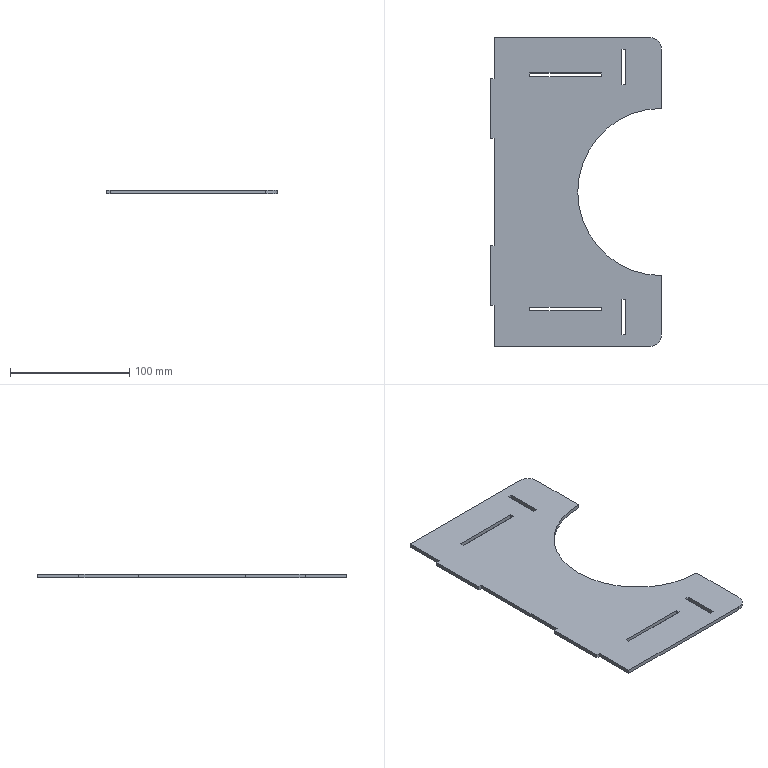Part | SolidWorks | features FlatPattern 1, SMBaseFlange 1, SheetMetal 1 | 1 solid | 34 faces | box 143.5 x 260 x 3.2 mm | volume 91069 mm3 | plane 31 | cylinder 3 | commonest cylinder face diameters 20 x2 140.5 x1
STEP:
#1=CARTESIAN_POINT('',(140.5,109.865,0.));
#2=VERTEX_POINT('',#1);
#3=CARTESIAN_POINT('',(130.5,119.865,0.));
#4=VERTEX_POINT('',#3);
#5=CARTESIAN_POINT('',(130.5,109.865,0.));
#6=DIRECTION('',(0.,0.,1.));
#7=DIRECTION('',(-1.,0.,0.));
#8=AXIS2_PLACEMENT_3D('',#5,#6,#7);
#9=CIRCLE('',#8,10.);
#10=EDGE_CURVE('',#2,#4,#9,.T.);
#11=ORIENTED_EDGE('',*,*,#10,.F.);
#12=CARTESIAN_POINT('',(140.5,109.865,-3.2));
#13=VERTEX_POINT('',#12);
#14=CARTESIAN_POINT('',(140.5,109.865,-3.2));
#15=DIRECTION('',(0.,0.,1.));
#16=VECTOR('',#15,1000.);
#17=LINE('',#14,#16);
#18=EDGE_CURVE('',#13,#2,#17,.T.);
#19=ORIENTED_EDGE('',*,*,#18,.F.);
#20=CARTESIAN_POINT('',(130.5,119.865,-3.2));
#21=VERTEX_POINT('',#20);
#22=CARTESIAN_POINT('',(130.5,109.865,-3.2));
#23=DIRECTION('',(0.,0.,1.));
#24=DIRECTION('',(-1.,0.,0.));
#25=AXIS2_PLACEMENT_3D('',#22,#23,#24);
#26=CIRCLE('',#25,10.);
#27=EDGE_CURVE('',#13,#21,#26,.T.);
#28=ORIENTED_EDGE('',*,*,#27,.T.);
#29=CARTESIAN_POINT('',(130.5,119.865,-3.2));
#30=DIRECTION('',(0.,0.,1.));
#31=VECTOR('',#30,1000.);
#32=LINE('',#29,#31);
#33=EDGE_CURVE('',#21,#4,#32,.T.);
#34=ORIENTED_EDGE('',*,*,#33,.T.);
#35=EDGE_LOOP('',(#11,#19,#28,#34));
#36=FACE_OUTER_BOUND('',#35,.T.);
#37=CARTESIAN_POINT('',(130.5,109.865,-3.2));
#38=DIRECTION('',(0.,0.,1.));
#39=DIRECTION('',(1.,0.,0.));
#40=AXIS2_PLACEMENT_3D('',#37,#38,#39);
#41=CYLINDRICAL_SURFACE('',#40,10.);
#42=ADVANCED_FACE('',(#36),#41,.T.);
#43=CARTESIAN_POINT('',(140.5,60.115,0.));
#44=VERTEX_POINT('',#43);
#45=CARTESIAN_POINT('',(140.5,109.865,0.));
#46=DIRECTION('',(0.,1.,0.));
#47=VECTOR('',#46,1000.);
#48=LINE('',#45,#47);
#49=EDGE_CURVE('',#44,#2,#48,.T.);
#50=ORIENTED_EDGE('',*,*,#49,.F.);
#51=CARTESIAN_POINT('',(140.5,60.115,-3.2));
#52=VERTEX_POINT('',#51);
#53=CARTESIAN_POINT('',(140.5,60.115,-3.2));
#54=DIRECTION('',(0.,0.,1.));
#55=VECTOR('',#54,1000.);
#56=LINE('',#53,#55);
#57=EDGE_CURVE('',#52,#44,#56,.T.);
#58=ORIENTED_EDGE('',*,*,#57,.F.);
#59=CARTESIAN_POINT('',(140.5,109.865,-3.2));
#60=DIRECTION('',(0.,1.,0.));
#61=VECTOR('',#60,1000.);
#62=LINE('',#59,#61);
#63=EDGE_CURVE('',#52,#13,#62,.T.);
#64=ORIENTED_EDGE('',*,*,#63,.T.);
#65=ORIENTED_EDGE('',*,*,#18,.T.);
#66=EDGE_LOOP('',(#50,#58,#64,#65));
#67=FACE_OUTER_BOUND('',#66,.T.);
#68=CARTESIAN_POINT('',(140.5,109.865,-3.2));
#69=DIRECTION('',(1.,0.,0.));
#70=DIRECTION('',(0.,0.,-1.));
#71=AXIS2_PLACEMENT_3D('',#68,#69,#70);
#72=PLANE('',#71);
#73=ADVANCED_FACE('',(#67),#72,.T.);
#74=CARTESIAN_POINT('',(140.5,-80.385,0.));
#75=VERTEX_POINT('',#74);
#76=CARTESIAN_POINT('',(140.5,-10.135,0.));
#77=DIRECTION('',(0.,0.,-1.));
#78=DIRECTION('',(1.,0.,0.));
#79=AXIS2_PLACEMENT_3D('',#76,#77,#78);
#80=CIRCLE('',#79,70.25);
#81=EDGE_CURVE('',#75,#44,#80,.T.);
#82=ORIENTED_EDGE('',*,*,#81,.F.);
#83=CARTESIAN_POINT('',(140.5,-80.385,-3.2));
#84=VERTEX_POINT('',#83);
#85=CARTESIAN_POINT('',(140.5,-80.385,-3.2));
#86=DIRECTION('',(0.,0.,1.));
#87=VECTOR('',#86,1000.);
#88=LINE('',#85,#87);
#89=EDGE_CURVE('',#84,#75,#88,.T.);
#90=ORIENTED_EDGE('',*,*,#89,.F.);
#91=CARTESIAN_POINT('',(140.5,-10.135,-3.2));
#92=DIRECTION('',(0.,0.,-1.));
#93=DIRECTION('',(1.,0.,0.));
#94=AXIS2_PLACEMENT_3D('',#91,#92,#93);
#95=CIRCLE('',#94,70.25);
#96=EDGE_CURVE('',#84,#52,#95,.T.);
#97=ORIENTED_EDGE('',*,*,#96,.T.);
#98=ORIENTED_EDGE('',*,*,#57,.T.);
#99=EDGE_LOOP('',(#82,#90,#97,#98));
#100=FACE_OUTER_BOUND('',#99,.T.);
#101=CARTESIAN_POINT('',(140.5,-10.135,-3.2));
#102=DIRECTION('',(0.,0.,1.));
#103=DIRECTION('',(1.,0.,0.));
#104=AXIS2_PLACEMENT_3D('',#101,#102,#103);
#105=CYLINDRICAL_SURFACE('',#104,70.25);
#106=ADVANCED_FACE('',(#100),#105,.F.);
#107=CARTESIAN_POINT('',(140.5,-130.135,0.));
#108=VERTEX_POINT('',#107);
#109=CARTESIAN_POINT('',(140.5,-80.385,0.));
#110=DIRECTION('',(0.,1.,0.));
#111=VECTOR('',#110,1000.);
#112=LINE('',#109,#111);
#113=EDGE_CURVE('',#108,#75,#112,.T.);
#114=ORIENTED_EDGE('',*,*,#113,.F.);
#115=CARTESIAN_POINT('',(140.5,-130.135,-3.2));
#116=VERTEX_POINT('',#115);
#117=CARTESIAN_POINT('',(140.5,-130.135,-3.2));
#118=DIRECTION('',(0.,0.,1.));
#119=VECTOR('',#118,1000.);
#120=LINE('',#117,#119);
#121=EDGE_CURVE('',#116,#108,#120,.T.);
#122=ORIENTED_EDGE('',*,*,#121,.F.);
#123=CARTESIAN_POINT('',(140.5,-80.385,-3.2));
#124=DIRECTION('',(0.,1.,0.));
#125=VECTOR('',#124,1000.);
#126=LINE('',#123,#125);
#127=EDGE_CURVE('',#116,#84,#126,.T.);
#128=ORIENTED_EDGE('',*,*,#127,.T.);
#129=ORIENTED_EDGE('',*,*,#89,.T.);
#130=EDGE_LOOP('',(#114,#122,#128,#129));
#131=FACE_OUTER_BOUND('',#130,.T.);
#132=CARTESIAN_POINT('',(140.5,-80.385,-3.2));
#133=DIRECTION('',(1.,0.,0.));
#134=DIRECTION('',(0.,0.,-1.));
#135=AXIS2_PLACEMENT_3D('',#132,#133,#134);
#136=PLANE('',#135);
#137=ADVANCED_FACE('',(#131),#136,.T.);
#138=CARTESIAN_POINT('',(130.5,-140.135,0.));
#139=VERTEX_POINT('',#138);
#140=CARTESIAN_POINT('',(130.5,-130.135,0.));
#141=DIRECTION('',(0.,0.,1.));
#142=DIRECTION('',(-1.,0.,0.));
#143=AXIS2_PLACEMENT_3D('',#140,#141,#142);
#144=CIRCLE('',#143,10.);
#145=EDGE_CURVE('',#139,#108,#144,.T.);
#146=ORIENTED_EDGE('',*,*,#145,.F.);
#147=CARTESIAN_POINT('',(130.5,-140.135,-3.2));
#148=VERTEX_POINT('',#147);
#149=CARTESIAN_POINT('',(130.5,-140.135,-3.2));
#150=DIRECTION('',(0.,0.,1.));
#151=VECTOR('',#150,1000.);
#152=LINE('',#149,#151);
#153=EDGE_CURVE('',#148,#139,#152,.T.);
#154=ORIENTED_EDGE('',*,*,#153,.F.);
#155=CARTESIAN_POINT('',(130.5,-130.135,-3.2));
#156=DIRECTION('',(0.,0.,1.));
#157=DIRECTION('',(-1.,0.,0.));
#158=AXIS2_PLACEMENT_3D('',#155,#156,#157);
#159=CIRCLE('',#158,10.);
#160=EDGE_CURVE('',#148,#116,#159,.T.);
#161=ORIENTED_EDGE('',*,*,#160,.T.);
#162=ORIENTED_EDGE('',*,*,#121,.T.);
#163=EDGE_LOOP('',(#146,#154,#161,#162));
#164=FACE_OUTER_BOUND('',#163,.T.);
#165=CARTESIAN_POINT('',(130.5,-130.135,-3.2));
#166=DIRECTION('',(0.,0.,1.));
#167=DIRECTION('',(1.,0.,0.));
#168=AXIS2_PLACEMENT_3D('',#165,#166,#167);
#169=CYLINDRICAL_SURFACE('',#168,10.);
#170=ADVANCED_FACE('',(#164),#169,.T.);
#171=CARTESIAN_POINT('',(0.,-140.135,0.));
#172=VERTEX_POINT('',#171);
#173=CARTESIAN_POINT('',(130.5,-140.135,0.));
#174=DIRECTION('',(1.,0.,0.));
#175=VECTOR('',#174,1000.);
#176=LINE('',#173,#175);
#177=EDGE_CURVE('',#172,#139,#176,.T.);
#178=ORIENTED_EDGE('',*,*,#177,.F.);
#179=CARTESIAN_POINT('',(0.,-140.135,-3.2));
#180=VERTEX_POINT('',#179);
#181=CARTESIAN_POINT('',(0.,-140.135,-3.2));
#182=DIRECTION('',(0.,0.,1.));
#183=VECTOR('',#182,1000.);
#184=LINE('',#181,#183);
#185=EDGE_CURVE('',#180,#172,#184,.T.);
#186=ORIENTED_EDGE('',*,*,#185,.F.);
#187=CARTESIAN_POINT('',(130.5,-140.135,-3.2));
#188=DIRECTION('',(1.,0.,0.));
#189=VECTOR('',#188,1000.);
#190=LINE('',#187,#189);
#191=EDGE_CURVE('',#180,#148,#190,.T.);
#192=ORIENTED_EDGE('',*,*,#191,.T.);
#193=ORIENTED_EDGE('',*,*,#153,.T.);
#194=EDGE_LOOP('',(#178,#186,#192,#193));
#195=FACE_OUTER_BOUND('',#194,.T.);
#196=CARTESIAN_POINT('',(130.5,-140.135,-3.2));
#197=DIRECTION('',(0.,-1.,0.));
#198=DIRECTION('',(0.,0.,-1.));
#199=AXIS2_PLACEMENT_3D('',#196,#197,#198);
#200=PLANE('',#199);
#201=ADVANCED_FACE('',(#195),#200,.T.);
#202=CARTESIAN_POINT('',(0.,-105.135,0.));
#203=VERTEX_POINT('',#202);
#204=CARTESIAN_POINT('',(0.,-140.135,0.));
#205=DIRECTION('',(0.,-1.,0.));
#206=VECTOR('',#205,1000.);
#207=LINE('',#204,#206);
#208=EDGE_CURVE('',#203,#172,#207,.T.);
#209=ORIENTED_EDGE('',*,*,#208,.F.);
#210=CARTESIAN_POINT('',(0.,-105.135,-3.2));
#211=VERTEX_POINT('',#210);
#212=CARTESIAN_POINT('',(0.,-105.135,-3.2));
#213=DIRECTION('',(0.,0.,1.));
#214=VECTOR('',#213,1000.);
#215=LINE('',#212,#214);
#216=EDGE_CURVE('',#211,#203,#215,.T.);
#217=ORIENTED_EDGE('',*,*,#216,.F.);
#218=CARTESIAN_POINT('',(0.,-140.135,-3.2));
#219=DIRECTION('',(0.,-1.,0.));
#220=VECTOR('',#219,1000.);
#221=LINE('',#218,#220);
#222=EDGE_CURVE('',#211,#180,#221,.T.);
#223=ORIENTED_EDGE('',*,*,#222,.T.);
#224=ORIENTED_EDGE('',*,*,#185,.T.);
#225=EDGE_LOOP('',(#209,#217,#223,#224));
#226=FACE_OUTER_BOUND('',#225,.T.);
#227=CARTESIAN_POINT('',(0.,-140.135,-3.2));
#228=DIRECTION('',(-1.,0.,0.));
#229=DIRECTION('',(0.,0.,1.));
#230=AXIS2_PLACEMENT_3D('',#227,#228,#229);
#231=PLANE('',#230);
#232=ADVANCED_FACE('',(#226),#231,.T.);
#233=CARTESIAN_POINT('',(-3.,-105.135,0.));
#234=VERTEX_POINT('',#233);
#235=CARTESIAN_POINT('',(0.,-105.135,0.));
#236=DIRECTION('',(1.,0.,0.));
#237=VECTOR('',#236,1000.);
#238=LINE('',#235,#237);
#239=EDGE_CURVE('',#234,#203,#238,.T.);
#240=ORIENTED_EDGE('',*,*,#239,.F.);
#241=CARTESIAN_POINT('',(-3.,-105.135,-3.2));
#242=VERTEX_POINT('',#241);
#243=CARTESIAN_POINT('',(-3.,-105.135,-3.2));
#244=DIRECTION('',(0.,0.,1.));
#245=VECTOR('',#244,1000.);
#246=LINE('',#243,#245);
#247=EDGE_CURVE('',#242,#234,#246,.T.);
#248=ORIENTED_EDGE('',*,*,#247,.F.);
#249=CARTESIAN_POINT('',(0.,-105.135,-3.2));
#250=DIRECTION('',(1.,0.,0.));
#251=VECTOR('',#250,1000.);
#252=LINE('',#249,#251);
#253=EDGE_CURVE('',#242,#211,#252,.T.);
#254=ORIENTED_EDGE('',*,*,#253,.T.);
#255=ORIENTED_EDGE('',*,*,#216,.T.);
#256=EDGE_LOOP('',(#240,#248,#254,#255));
#257=FACE_OUTER_BOUND('',#256,.T.);
#258=CARTESIAN_POINT('',(0.,-105.135,-3.2));
#259=DIRECTION('',(0.,-1.,0.));
#260=DIRECTION('',(0.,0.,-1.));
#261=AXIS2_PLACEMENT_3D('',#258,#259,#260);
#262=PLANE('',#261);
#263=ADVANCED_FACE('',(#257),#262,.T.);
#264=CARTESIAN_POINT('',(-3.,-55.135,0.));
#265=VERTEX_POINT('',#264);
#266=CARTESIAN_POINT('',(-3.,-105.135,0.));
#267=DIRECTION('',(0.,-1.,0.));
#268=VECTOR('',#267,1000.);
#269=LINE('',#266,#268);
#270=EDGE_CURVE('',#265,#234,#269,.T.);
#271=ORIENTED_EDGE('',*,*,#270,.F.);
#272=CARTESIAN_POINT('',(-3.,-55.135,-3.2));
#273=VERTEX_POINT('',#272);
#274=CARTESIAN_POINT('',(-3.,-55.135,-3.2));
#275=DIRECTION('',(0.,0.,1.));
#276=VECTOR('',#275,1000.);
#277=LINE('',#274,#276);
#278=EDGE_CURVE('',#273,#265,#277,.T.);
#279=ORIENTED_EDGE('',*,*,#278,.F.);
#280=CARTESIAN_POINT('',(-3.,-105.135,-3.2));
#281=DIRECTION('',(0.,-1.,0.));
#282=VECTOR('',#281,1000.);
#283=LINE('',#280,#282);
#284=EDGE_CURVE('',#273,#242,#283,.T.);
#285=ORIENTED_EDGE('',*,*,#284,.T.);
#286=ORIENTED_EDGE('',*,*,#247,.T.);
#287=EDGE_LOOP('',(#271,#279,#285,#286));
#288=FACE_OUTER_BOUND('',#287,.T.);
#289=CARTESIAN_POINT('',(-3.,-105.135,-3.2));
#290=DIRECTION('',(-1.,0.,0.));
#291=DIRECTION('',(0.,-1.,0.));
#292=AXIS2_PLACEMENT_3D('',#289,#290,#291);
#293=PLANE('',#292);
#294=ADVANCED_FACE('',(#288),#293,.T.);
#295=CARTESIAN_POINT('',(0.,-55.135,0.));
#296=VERTEX_POINT('',#295);
#297=CARTESIAN_POINT('',(-3.,-55.135,0.));
#298=DIRECTION('',(-1.,0.,0.));
#299=VECTOR('',#298,1000.);
#300=LINE('',#297,#299);
#301=EDGE_CURVE('',#296,#265,#300,.T.);
#302=ORIENTED_EDGE('',*,*,#301,.F.);
#303=CARTESIAN_POINT('',(0.,-55.135,-3.2));
#304=VERTEX_POINT('',#303);
#305=CARTESIAN_POINT('',(0.,-55.135,-3.2));
#306=DIRECTION('',(0.,0.,1.));
#307=VECTOR('',#306,1000.);
#308=LINE('',#305,#307);
#309=EDGE_CURVE('',#304,#296,#308,.T.);
#310=ORIENTED_EDGE('',*,*,#309,.F.);
#311=CARTESIAN_POINT('',(-3.,-55.135,-3.2));
#312=DIRECTION('',(-1.,0.,0.));
#313=VECTOR('',#312,1000.);
#314=LINE('',#311,#313);
#315=EDGE_CURVE('',#304,#273,#314,.T.);
#316=ORIENTED_EDGE('',*,*,#315,.T.);
#317=ORIENTED_EDGE('',*,*,#278,.T.);
#318=EDGE_LOOP('',(#302,#310,#316,#317));
#319=FACE_OUTER_BOUND('',#318,.T.);
#320=CARTESIAN_POINT('',(-3.,-55.135,-3.2));
#321=DIRECTION('',(0.,1.,0.));
#322=DIRECTION('',(0.,0.,1.));
#323=AXIS2_PLACEMENT_3D('',#320,#321,#322);
#324=PLANE('',#323);
#325=ADVANCED_FACE('',(#319),#324,.T.);
#326=CARTESIAN_POINT('',(0.,34.865,0.));
#327=VERTEX_POINT('',#326);
#328=CARTESIAN_POINT('',(0.,-55.135,0.));
#329=DIRECTION('',(0.,-1.,0.));
#330=VECTOR('',#329,1000.);
#331=LINE('',#328,#330);
#332=EDGE_CURVE('',#327,#296,#331,.T.);
#333=ORIENTED_EDGE('',*,*,#332,.F.);
#334=CARTESIAN_POINT('',(0.,34.865,-3.2));
#335=VERTEX_POINT('',#334);
#336=CARTESIAN_POINT('',(0.,34.865,-3.2));
#337=DIRECTION('',(0.,0.,1.));
#338=VECTOR('',#337,1000.);
#339=LINE('',#336,#338);
#340=EDGE_CURVE('',#335,#327,#339,.T.);
#341=ORIENTED_EDGE('',*,*,#340,.F.);
#342=CARTESIAN_POINT('',(0.,-55.135,-3.2));
#343=DIRECTION('',(0.,-1.,0.));
#344=VECTOR('',#343,1000.);
#345=LINE('',#342,#344);
#346=EDGE_CURVE('',#335,#304,#345,.T.);
#347=ORIENTED_EDGE('',*,*,#346,.T.);
#348=ORIENTED_EDGE('',*,*,#309,.T.);
#349=EDGE_LOOP('',(#333,#341,#347,#348));
#350=FACE_OUTER_BOUND('',#349,.T.);
#351=CARTESIAN_POINT('',(0.,-55.135,-3.2));
#352=DIRECTION('',(-1.,0.,0.));
#353=DIRECTION('',(0.,0.,1.));
#354=AXIS2_PLACEMENT_3D('',#351,#352,#353);
#355=PLANE('',#354);
#356=ADVANCED_FACE('',(#350),#355,.T.);
#357=CARTESIAN_POINT('',(-3.,34.865,0.));
#358=VERTEX_POINT('',#357);
#359=CARTESIAN_POINT('',(-3.,34.865,0.));
#360=DIRECTION('',(1.,0.,0.));
#361=VECTOR('',#360,1000.);
#362=LINE('',#359,#361);
#363=EDGE_CURVE('',#358,#327,#362,.T.);
#364=ORIENTED_EDGE('',*,*,#363,.F.);
#365=CARTESIAN_POINT('',(-3.,34.865,-3.2));
#366=VERTEX_POINT('',#365);
#367=CARTESIAN_POINT('',(-3.,34.865,-3.2));
#368=DIRECTION('',(0.,0.,1.));
#369=VECTOR('',#368,1000.);
#370=LINE('',#367,#369);
#371=EDGE_CURVE('',#366,#358,#370,.T.);
#372=ORIENTED_EDGE('',*,*,#371,.F.);
#373=CARTESIAN_POINT('',(-3.,34.865,-3.2));
#374=DIRECTION('',(1.,0.,0.));
#375=VECTOR('',#374,1000.);
#376=LINE('',#373,#375);
#377=EDGE_CURVE('',#366,#335,#376,.T.);
#378=ORIENTED_EDGE('',*,*,#377,.T.);
#379=ORIENTED_EDGE('',*,*,#340,.T.);
#380=EDGE_LOOP('',(#364,#372,#378,#379));
#381=FACE_OUTER_BOUND('',#380,.T.);
#382=CARTESIAN_POINT('',(-3.,34.865,-3.2));
#383=DIRECTION('',(0.,-1.,0.));
#384=DIRECTION('',(0.,0.,-1.));
#385=AXIS2_PLACEMENT_3D('',#382,#383,#384);
#386=PLANE('',#385);
#387=ADVANCED_FACE('',(#381),#386,.T.);
#388=CARTESIAN_POINT('',(-3.,84.865,0.));
#389=VERTEX_POINT('',#388);
#390=CARTESIAN_POINT('',(-3.,84.865,0.));
#391=DIRECTION('',(0.,-1.,0.));
#392=VECTOR('',#391,1000.);
#393=LINE('',#390,#392);
#394=EDGE_CURVE('',#389,#358,#393,.T.);
#395=ORIENTED_EDGE('',*,*,#394,.F.);
#396=CARTESIAN_POINT('',(-3.,84.865,-3.2));
#397=VERTEX_POINT('',#396);
#398=CARTESIAN_POINT('',(-3.,84.865,-3.2));
#399=DIRECTION('',(0.,0.,1.));
#400=VECTOR('',#399,1000.);
#401=LINE('',#398,#400);
#402=EDGE_CURVE('',#397,#389,#401,.T.);
#403=ORIENTED_EDGE('',*,*,#402,.F.);
#404=CARTESIAN_POINT('',(-3.,84.865,-3.2));
#405=DIRECTION('',(0.,-1.,0.));
#406=VECTOR('',#405,1000.);
#407=LINE('',#404,#406);
#408=EDGE_CURVE('',#397,#366,#407,.T.);
#409=ORIENTED_EDGE('',*,*,#408,.T.);
#410=ORIENTED_EDGE('',*,*,#371,.T.);
#411=EDGE_LOOP('',(#395,#403,#409,#410));
#412=FACE_OUTER_BOUND('',#411,.T.);
#413=CARTESIAN_POINT('',(-3.,84.865,-3.2));
#414=DIRECTION('',(-1.,0.,0.));
#415=DIRECTION('',(0.,-1.,0.));
#416=AXIS2_PLACEMENT_3D('',#413,#414,#415);
#417=PLANE('',#416);
#418=ADVANCED_FACE('',(#412),#417,.T.);
#419=CARTESIAN_POINT('',(0.,84.865,0.));
#420=VERTEX_POINT('',#419);
#421=CARTESIAN_POINT('',(0.,84.865,0.));
#422=DIRECTION('',(-1.,0.,0.));
#423=VECTOR('',#422,1000.);
#424=LINE('',#421,#423);
#425=EDGE_CURVE('',#420,#389,#424,.T.);
#426=ORIENTED_EDGE('',*,*,#425,.F.);
#427=CARTESIAN_POINT('',(0.,84.865,-3.2));
#428=VERTEX_POINT('',#427);
#429=CARTESIAN_POINT('',(0.,84.865,-3.2));
#430=DIRECTION('',(0.,0.,1.));
#431=VECTOR('',#430,1000.);
#432=LINE('',#429,#431);
#433=EDGE_CURVE('',#428,#420,#432,.T.);
#434=ORIENTED_EDGE('',*,*,#433,.F.);
#435=CARTESIAN_POINT('',(0.,84.865,-3.2));
#436=DIRECTION('',(-1.,0.,0.));
#437=VECTOR('',#436,1000.);
#438=LINE('',#435,#437);
#439=EDGE_CURVE('',#428,#397,#438,.T.);
#440=ORIENTED_EDGE('',*,*,#439,.T.);
#441=ORIENTED_EDGE('',*,*,#402,.T.);
#442=EDGE_LOOP('',(#426,#434,#440,#441));
#443=FACE_OUTER_BOUND('',#442,.T.);
#444=CARTESIAN_POINT('',(0.,84.865,-3.2));
#445=DIRECTION('',(0.,1.,0.));
#446=DIRECTION('',(-1.,0.,0.));
#447=AXIS2_PLACEMENT_3D('',#444,#445,#446);
#448=PLANE('',#447);
#449=ADVANCED_FACE('',(#443),#448,.T.);
#450=CARTESIAN_POINT('',(0.,119.865,0.));
#451=VERTEX_POINT('',#450);
#452=CARTESIAN_POINT('',(0.,84.865,0.));
#453=DIRECTION('',(0.,-1.,0.));
#454=VECTOR('',#453,1000.);
#455=LINE('',#452,#454);
#456=EDGE_CURVE('',#451,#420,#455,.T.);
#457=ORIENTED_EDGE('',*,*,#456,.F.);
#458=CARTESIAN_POINT('',(0.,119.865,-3.2));
#459=VERTEX_POINT('',#458);
#460=CARTESIAN_POINT('',(0.,119.865,-3.2));
#461=DIRECTION('',(0.,0.,1.));
#462=VECTOR('',#461,1000.);
#463=LINE('',#460,#462);
#464=EDGE_CURVE('',#459,#451,#463,.T.);
#465=ORIENTED_EDGE('',*,*,#464,.F.);
#466=CARTESIAN_POINT('',(0.,84.865,-3.2));
#467=DIRECTION('',(0.,-1.,0.));
#468=VECTOR('',#467,1000.);
#469=LINE('',#466,#468);
#470=EDGE_CURVE('',#459,#428,#469,.T.);
#471=ORIENTED_EDGE('',*,*,#470,.T.);
#472=ORIENTED_EDGE('',*,*,#433,.T.);
#473=EDGE_LOOP('',(#457,#465,#471,#472));
#474=FACE_OUTER_BOUND('',#473,.T.);
#475=CARTESIAN_POINT('',(0.,84.865,-3.2));
#476=DIRECTION('',(-1.,0.,0.));
#477=DIRECTION('',(0.,0.,1.));
#478=AXIS2_PLACEMENT_3D('',#475,#476,#477);
#479=PLANE('',#478);
#480=ADVANCED_FACE('',(#474),#479,.T.);
#481=CARTESIAN_POINT('',(0.,119.865,0.));
#482=DIRECTION('',(-1.,0.,0.));
#483=VECTOR('',#482,1000.);
#484=LINE('',#481,#483);
#485=EDGE_CURVE('',#4,#451,#484,.T.);
#486=ORIENTED_EDGE('',*,*,#485,.F.);
#487=ORIENTED_EDGE('',*,*,#33,.F.);
#488=CARTESIAN_POINT('',(0.,119.865,-3.2));
#489=DIRECTION('',(-1.,0.,0.));
#490=VECTOR('',#489,1000.);
#491=LINE('',#488,#490);
#492=EDGE_CURVE('',#21,#459,#491,.T.);
#493=ORIENTED_EDGE('',*,*,#492,.T.);
#494=ORIENTED_EDGE('',*,*,#464,.T.);
#495=EDGE_LOOP('',(#486,#487,#493,#494));
#496=FACE_OUTER_BOUND('',#495,.T.);
#497=CARTESIAN_POINT('',(0.,119.865,-3.2));
#498=DIRECTION('',(0.,1.,0.));
#499=DIRECTION('',(-1.,0.,0.));
#500=AXIS2_PLACEMENT_3D('',#497,#498,#499);
#501=PLANE('',#500);
#502=ADVANCED_FACE('',(#496),#501,.T.);
#503=CARTESIAN_POINT('',(110.5,-130.135,-3.2));
#504=VERTEX_POINT('',#503);
#505=CARTESIAN_POINT('',(110.5,-100.135,-3.2));
#506=VERTEX_POINT('',#505);
#507=CARTESIAN_POINT('',(110.5,-100.135,-3.2));
#508=DIRECTION('',(0.,1.,0.));
#509=VECTOR('',#508,1000.);
#510=LINE('',#507,#509);
#511=EDGE_CURVE('',#504,#506,#510,.T.);
#512=ORIENTED_EDGE('',*,*,#511,.T.);
#513=CARTESIAN_POINT('',(107.3,-100.135,-3.2));
#514=VERTEX_POINT('',#513);
#515=CARTESIAN_POINT('',(110.5,-100.135,-3.2));
#516=DIRECTION('',(-1.,0.,0.));
#517=VECTOR('',#516,1000.);
#518=LINE('',#515,#517);
#519=EDGE_CURVE('',#506,#514,#518,.T.);
#520=ORIENTED_EDGE('',*,*,#519,.T.);
#521=CARTESIAN_POINT('',(107.3,-130.135,-3.2));
#522=VERTEX_POINT('',#521);
#523=CARTESIAN_POINT('',(107.3,-100.135,-3.2));
#524=DIRECTION('',(0.,-1.,0.));
#525=VECTOR('',#524,1000.);
#526=LINE('',#523,#525);
#527=EDGE_CURVE('',#514,#522,#526,.T.);
#528=ORIENTED_EDGE('',*,*,#527,.T.);
#529=CARTESIAN_POINT('',(110.5,-130.135,-3.2));
#530=DIRECTION('',(1.,0.,0.));
#531=VECTOR('',#530,1000.);
#532=LINE('',#529,#531);
#533=EDGE_CURVE('',#522,#504,#532,.T.);
#534=ORIENTED_EDGE('',*,*,#533,.T.);
#535=EDGE_LOOP('',(#512,#520,#528,#534));
#536=FACE_BOUND('',#535,.T.);
#537=CARTESIAN_POINT('',(107.3,109.865,-3.2));
#538=VERTEX_POINT('',#537);
#539=CARTESIAN_POINT('',(107.3,79.865,-3.2));
#540=VERTEX_POINT('',#539);
#541=CARTESIAN_POINT('',(107.3,79.865,-3.2));
#542=DIRECTION('',(0.,-1.,0.));
#543=VECTOR('',#542,1000.);
#544=LINE('',#541,#543);
#545=EDGE_CURVE('',#538,#540,#544,.T.);
#546=ORIENTED_EDGE('',*,*,#545,.T.);
#547=CARTESIAN_POINT('',(110.5,79.865,-3.2));
#548=VERTEX_POINT('',#547);
#549=CARTESIAN_POINT('',(107.3,79.865,-3.2));
#550=DIRECTION('',(1.,0.,0.));
#551=VECTOR('',#550,1000.);
#552=LINE('',#549,#551);
#553=EDGE_CURVE('',#540,#548,#552,.T.);
#554=ORIENTED_EDGE('',*,*,#553,.T.);
#555=CARTESIAN_POINT('',(110.5,109.865,-3.2));
#556=VERTEX_POINT('',#555);
#557=CARTESIAN_POINT('',(110.5,79.865,-3.2));
#558=DIRECTION('',(0.,1.,0.));
#559=VECTOR('',#558,1000.);
#560=LINE('',#557,#559);
#561=EDGE_CURVE('',#548,#556,#560,.T.);
#562=ORIENTED_EDGE('',*,*,#561,.T.);
#563=CARTESIAN_POINT('',(107.3,109.865,-3.2));
#564=DIRECTION('',(-1.,0.,0.));
#565=VECTOR('',#564,1000.);
#566=LINE('',#563,#565);
#567=EDGE_CURVE('',#556,#538,#566,.T.);
#568=ORIENTED_EDGE('',*,*,#567,.T.);
#569=EDGE_LOOP('',(#546,#554,#562,#568));
#570=FACE_BOUND('',#569,.T.);
#571=CARTESIAN_POINT('',(90.,-110.135,-3.2));
#572=VERTEX_POINT('',#571);
#573=CARTESIAN_POINT('',(90.,-106.935,-3.2));
#574=VERTEX_POINT('',#573);
#575=CARTESIAN_POINT('',(90.,-106.935,-3.2));
#576=DIRECTION('',(0.,1.,0.));
#577=VECTOR('',#576,1000.);
#578=LINE('',#575,#577);
#579=EDGE_CURVE('',#572,#574,#578,.T.);
#580=ORIENTED_EDGE('',*,*,#579,.T.);
#581=CARTESIAN_POINT('',(30.,-106.935,-3.2));
#582=VERTEX_POINT('',#581);
#583=CARTESIAN_POINT('',(90.,-106.935,-3.2));
#584=DIRECTION('',(-1.,0.,0.));
#585=VECTOR('',#584,1000.);
#586=LINE('',#583,#585);
#587=EDGE_CURVE('',#574,#582,#586,.T.);
#588=ORIENTED_EDGE('',*,*,#587,.T.);
#589=CARTESIAN_POINT('',(30.,-110.135,-3.2));
#590=VERTEX_POINT('',#589);
#591=CARTESIAN_POINT('',(30.,-106.935,-3.2));
#592=DIRECTION('',(0.,-1.,0.));
#593=VECTOR('',#592,1000.);
#594=LINE('',#591,#593);
#595=EDGE_CURVE('',#582,#590,#594,.T.);
#596=ORIENTED_EDGE('',*,*,#595,.T.);
#597=CARTESIAN_POINT('',(90.,-110.135,-3.2));
#598=DIRECTION('',(1.,0.,0.));
#599=VECTOR('',#598,1000.);
#600=LINE('',#597,#599);
#601=EDGE_CURVE('',#590,#572,#600,.T.);
#602=ORIENTED_EDGE('',*,*,#601,.T.);
#603=EDGE_LOOP('',(#580,#588,#596,#602));
#604=FACE_BOUND('',#603,.T.);
#605=CARTESIAN_POINT('',(90.,86.665,-3.2));
#606=VERTEX_POINT('',#605);
#607=CARTESIAN_POINT('',(90.,89.865,-3.2));
#608=VERTEX_POINT('',#607);
#609=CARTESIAN_POINT('',(90.,89.865,-3.2));
#610=DIRECTION('',(0.,1.,0.));
#611=VECTOR('',#610,1000.);
#612=LINE('',#609,#611);
#613=EDGE_CURVE('',#606,#608,#612,.T.);
#614=ORIENTED_EDGE('',*,*,#613,.T.);
#615=CARTESIAN_POINT('',(30.,89.865,-3.2));
#616=VERTEX_POINT('',#615);
#617=CARTESIAN_POINT('',(90.,89.865,-3.2));
#618=DIRECTION('',(-1.,0.,0.));
#619=VECTOR('',#618,1000.);
#620=LINE('',#617,#619);
#621=EDGE_CURVE('',#608,#616,#620,.T.);
#622=ORIENTED_EDGE('',*,*,#621,.T.);
#623=CARTESIAN_POINT('',(30.,86.665,-3.2));
#624=VERTEX_POINT('',#623);
#625=CARTESIAN_POINT('',(30.,89.865,-3.2));
#626=DIRECTION('',(0.,-1.,0.));
#627=VECTOR('',#626,1000.);
#628=LINE('',#625,#627);
#629=EDGE_CURVE('',#616,#624,#628,.T.);
#630=ORIENTED_EDGE('',*,*,#629,.T.);
#631=CARTESIAN_POINT('',(90.,86.665,-3.2));
#632=DIRECTION('',(1.,0.,0.));
#633=VECTOR('',#632,1000.);
#634=LINE('',#631,#633);
#635=EDGE_CURVE('',#624,#606,#634,.T.);
#636=ORIENTED_EDGE('',*,*,#635,.T.);
#637=EDGE_LOOP('',(#614,#622,#630,#636));
#638=FACE_BOUND('',#637,.T.);
#639=ORIENTED_EDGE('',*,*,#27,.F.);
#640=ORIENTED_EDGE('',*,*,#63,.F.);
#641=ORIENTED_EDGE('',*,*,#96,.F.);
#642=ORIENTED_EDGE('',*,*,#127,.F.);
#643=ORIENTED_EDGE('',*,*,#160,.F.);
#644=ORIENTED_EDGE('',*,*,#191,.F.);
#645=ORIENTED_EDGE('',*,*,#222,.F.);
#646=ORIENTED_EDGE('',*,*,#253,.F.);
#647=ORIENTED_EDGE('',*,*,#284,.F.);
#648=ORIENTED_EDGE('',*,*,#315,.F.);
#649=ORIENTED_EDGE('',*,*,#346,.F.);
#650=ORIENTED_EDGE('',*,*,#377,.F.);
#651=ORIENTED_EDGE('',*,*,#408,.F.);
#652=ORIENTED_EDGE('',*,*,#439,.F.);
#653=ORIENTED_EDGE('',*,*,#470,.F.);
#654=ORIENTED_EDGE('',*,*,#492,.F.);
#655=EDGE_LOOP('',(#639,#640,#641,#642,#643,#644,#645,#646,#647,#648,#649,#650,#651,#652,#653,#654));
#656=FACE_OUTER_BOUND('',#655,.T.);
#657=CARTESIAN_POINT('',(130.5,109.865,-3.2));
#658=DIRECTION('',(0.,0.,-1.));
#659=DIRECTION('',(-1.,0.,0.));
#660=AXIS2_PLACEMENT_3D('',#657,#658,#659);
#661=PLANE('',#660);
#662=ADVANCED_FACE('',(#536,#570,#604,#638,#656),#661,.T.);
#663=CARTESIAN_POINT('',(110.5,-100.135,0.));
#664=VERTEX_POINT('',#663);
#665=CARTESIAN_POINT('',(107.3,-100.135,0.));
#666=VERTEX_POINT('',#665);
#667=CARTESIAN_POINT('',(110.5,-100.135,0.));
#668=DIRECTION('',(-1.,0.,0.));
#669=VECTOR('',#668,1000.);
#670=LINE('',#667,#669);
#671=EDGE_CURVE('',#664,#666,#670,.T.);
#672=ORIENTED_EDGE('',*,*,#671,.F.);
#673=CARTESIAN_POINT('',(110.5,-130.135,0.));
#674=VERTEX_POINT('',#673);
#675=CARTESIAN_POINT('',(110.5,-100.135,0.));
#676=DIRECTION('',(0.,1.,0.));
#677=VECTOR('',#676,1000.);
#678=LINE('',#675,#677);
#679=EDGE_CURVE('',#674,#664,#678,.T.);
#680=ORIENTED_EDGE('',*,*,#679,.F.);
#681=CARTESIAN_POINT('',(107.3,-130.135,0.));
#682=VERTEX_POINT('',#681);
#683=CARTESIAN_POINT('',(110.5,-130.135,0.));
#684=DIRECTION('',(1.,0.,0.));
#685=VECTOR('',#684,1000.);
#686=LINE('',#683,#685);
#687=EDGE_CURVE('',#682,#674,#686,.T.);
#688=ORIENTED_EDGE('',*,*,#687,.F.);
#689=CARTESIAN_POINT('',(107.3,-100.135,0.));
#690=DIRECTION('',(0.,-1.,0.));
#691=VECTOR('',#690,1000.);
#692=LINE('',#689,#691);
#693=EDGE_CURVE('',#666,#682,#692,.T.);
#694=ORIENTED_EDGE('',*,*,#693,.F.);
#695=EDGE_LOOP('',(#672,#680,#688,#694));
#696=FACE_BOUND('',#695,.T.);
#697=CARTESIAN_POINT('',(107.3,79.865,0.));
#698=VERTEX_POINT('',#697);
#699=CARTESIAN_POINT('',(110.5,79.865,0.));
#700=VERTEX_POINT('',#699);
#701=CARTESIAN_POINT('',(107.3,79.865,0.));
#702=DIRECTION('',(1.,0.,0.));
#703=VECTOR('',#702,1000.);
#704=LINE('',#701,#703);
#705=EDGE_CURVE('',#698,#700,#704,.T.);
#706=ORIENTED_EDGE('',*,*,#705,.F.);
#707=CARTESIAN_POINT('',(107.3,109.865,0.));
#708=VERTEX_POINT('',#707);
#709=CARTESIAN_POINT('',(107.3,79.865,0.));
#710=DIRECTION('',(0.,-1.,0.));
#711=VECTOR('',#710,1000.);
#712=LINE('',#709,#711);
#713=EDGE_CURVE('',#708,#698,#712,.T.);
#714=ORIENTED_EDGE('',*,*,#713,.F.);
#715=CARTESIAN_POINT('',(110.5,109.865,0.));
#716=VERTEX_POINT('',#715);
#717=CARTESIAN_POINT('',(107.3,109.865,0.));
#718=DIRECTION('',(-1.,0.,0.));
#719=VECTOR('',#718,1000.);
#720=LINE('',#717,#719);
#721=EDGE_CURVE('',#716,#708,#720,.T.);
#722=ORIENTED_EDGE('',*,*,#721,.F.);
#723=CARTESIAN_POINT('',(110.5,79.865,0.));
#724=DIRECTION('',(0.,1.,0.));
#725=VECTOR('',#724,1000.);
#726=LINE('',#723,#725);
#727=EDGE_CURVE('',#700,#716,#726,.T.);
#728=ORIENTED_EDGE('',*,*,#727,.F.);
#729=EDGE_LOOP('',(#706,#714,#722,#728));
#730=FACE_BOUND('',#729,.T.);
#731=CARTESIAN_POINT('',(90.,-106.935,0.));
#732=VERTEX_POINT('',#731);
#733=CARTESIAN_POINT('',(30.,-106.935,0.));
#734=VERTEX_POINT('',#733);
#735=CARTESIAN_POINT('',(90.,-106.935,0.));
#736=DIRECTION('',(-1.,0.,0.));
#737=VECTOR('',#736,1000.);
#738=LINE('',#735,#737);
#739=EDGE_CURVE('',#732,#734,#738,.T.);
#740=ORIENTED_EDGE('',*,*,#739,.F.);
#741=CARTESIAN_POINT('',(90.,-110.135,0.));
#742=VERTEX_POINT('',#741);
#743=CARTESIAN_POINT('',(90.,-106.935,0.));
#744=DIRECTION('',(0.,1.,0.));
#745=VECTOR('',#744,1000.);
#746=LINE('',#743,#745);
#747=EDGE_CURVE('',#742,#732,#746,.T.);
#748=ORIENTED_EDGE('',*,*,#747,.F.);
#749=CARTESIAN_POINT('',(30.,-110.135,0.));
#750=VERTEX_POINT('',#749);
#751=CARTESIAN_POINT('',(90.,-110.135,0.));
#752=DIRECTION('',(1.,0.,0.));
#753=VECTOR('',#752,1000.);
#754=LINE('',#751,#753);
#755=EDGE_CURVE('',#750,#742,#754,.T.);
#756=ORIENTED_EDGE('',*,*,#755,.F.);
#757=CARTESIAN_POINT('',(30.,-106.935,0.));
#758=DIRECTION('',(0.,-1.,0.));
#759=VECTOR('',#758,1000.);
#760=LINE('',#757,#759);
#761=EDGE_CURVE('',#734,#750,#760,.T.);
#762=ORIENTED_EDGE('',*,*,#761,.F.);
#763=EDGE_LOOP('',(#740,#748,#756,#762));
#764=FACE_BOUND('',#763,.T.);
#765=CARTESIAN_POINT('',(90.,89.865,0.));
#766=VERTEX_POINT('',#765);
#767=CARTESIAN_POINT('',(30.,89.865,0.));
#768=VERTEX_POINT('',#767);
#769=CARTESIAN_POINT('',(90.,89.865,0.));
#770=DIRECTION('',(-1.,0.,0.));
#771=VECTOR('',#770,1000.);
#772=LINE('',#769,#771);
#773=EDGE_CURVE('',#766,#768,#772,.T.);
#774=ORIENTED_EDGE('',*,*,#773,.F.);
#775=CARTESIAN_POINT('',(90.,86.665,0.));
#776=VERTEX_POINT('',#775);
#777=CARTESIAN_POINT('',(90.,89.865,0.));
#778=DIRECTION('',(0.,1.,0.));
#779=VECTOR('',#778,1000.);
#780=LINE('',#777,#779);
#781=EDGE_CURVE('',#776,#766,#780,.T.);
#782=ORIENTED_EDGE('',*,*,#781,.F.);
#783=CARTESIAN_POINT('',(30.,86.665,0.));
#784=VERTEX_POINT('',#783);
#785=CARTESIAN_POINT('',(90.,86.665,0.));
#786=DIRECTION('',(1.,0.,0.));
#787=VECTOR('',#786,1000.);
#788=LINE('',#785,#787);
#789=EDGE_CURVE('',#784,#776,#788,.T.);
#790=ORIENTED_EDGE('',*,*,#789,.F.);
#791=CARTESIAN_POINT('',(30.,89.865,0.));
#792=DIRECTION('',(0.,-1.,0.));
#793=VECTOR('',#792,1000.);
#794=LINE('',#791,#793);
#795=EDGE_CURVE('',#768,#784,#794,.T.);
#796=ORIENTED_EDGE('',*,*,#795,.F.);
#797=EDGE_LOOP('',(#774,#782,#790,#796));
#798=FACE_BOUND('',#797,.T.);
#799=ORIENTED_EDGE('',*,*,#10,.T.);
#800=ORIENTED_EDGE('',*,*,#485,.T.);
#801=ORIENTED_EDGE('',*,*,#456,.T.);
#802=ORIENTED_EDGE('',*,*,#425,.T.);
#803=ORIENTED_EDGE('',*,*,#394,.T.);
#804=ORIENTED_EDGE('',*,*,#363,.T.);
#805=ORIENTED_EDGE('',*,*,#332,.T.);
#806=ORIENTED_EDGE('',*,*,#301,.T.);
#807=ORIENTED_EDGE('',*,*,#270,.T.);
#808=ORIENTED_EDGE('',*,*,#239,.T.);
#809=ORIENTED_EDGE('',*,*,#208,.T.);
#810=ORIENTED_EDGE('',*,*,#177,.T.);
#811=ORIENTED_EDGE('',*,*,#145,.T.);
#812=ORIENTED_EDGE('',*,*,#113,.T.);
#813=ORIENTED_EDGE('',*,*,#81,.T.);
#814=ORIENTED_EDGE('',*,*,#49,.T.);
#815=EDGE_LOOP('',(#799,#800,#801,#802,#803,#804,#805,#806,#807,#808,#809,#810,#811,#812,#813,#814));
#816=FACE_OUTER_BOUND('',#815,.T.);
#817=CARTESIAN_POINT('',(130.5,109.865,0.));
#818=DIRECTION('',(0.,0.,-1.));
#819=DIRECTION('',(-1.,0.,0.));
#820=AXIS2_PLACEMENT_3D('',#817,#818,#819);
#821=PLANE('',#820);
#822=ADVANCED_FACE('',(#696,#730,#764,#798,#816),#821,.F.);
#823=ORIENTED_EDGE('',*,*,#781,.T.);
#824=CARTESIAN_POINT('',(90.,89.865,-3.2));
#825=DIRECTION('',(0.,0.,1.));
#826=VECTOR('',#825,1000.);
#827=LINE('',#824,#826);
#828=EDGE_CURVE('',#608,#766,#827,.T.);
#829=ORIENTED_EDGE('',*,*,#828,.F.);
#830=ORIENTED_EDGE('',*,*,#613,.F.);
#831=CARTESIAN_POINT('',(90.,86.665,-3.2));
#832=DIRECTION('',(0.,0.,1.));
#833=VECTOR('',#832,1000.);
#834=LINE('',#831,#833);
#835=EDGE_CURVE('',#606,#776,#834,.T.);
#836=ORIENTED_EDGE('',*,*,#835,.T.);
#837=EDGE_LOOP('',(#823,#829,#830,#836));
#838=FACE_OUTER_BOUND('',#837,.T.);
#839=CARTESIAN_POINT('',(90.,89.865,-3.2));
#840=DIRECTION('',(1.,0.,0.));
#841=DIRECTION('',(0.,0.,-1.));
#842=AXIS2_PLACEMENT_3D('',#839,#840,#841);
#843=PLANE('',#842);
#844=ADVANCED_FACE('',(#838),#843,.F.);
#845=ORIENTED_EDGE('',*,*,#789,.T.);
#846=ORIENTED_EDGE('',*,*,#835,.F.);
#847=ORIENTED_EDGE('',*,*,#635,.F.);
#848=CARTESIAN_POINT('',(30.,86.665,-3.2));
#849=DIRECTION('',(0.,0.,1.));
#850=VECTOR('',#849,1000.);
#851=LINE('',#848,#850);
#852=EDGE_CURVE('',#624,#784,#851,.T.);
#853=ORIENTED_EDGE('',*,*,#852,.T.);
#854=EDGE_LOOP('',(#845,#846,#847,#853));
#855=FACE_OUTER_BOUND('',#854,.T.);
#856=CARTESIAN_POINT('',(90.,86.665,-3.2));
#857=DIRECTION('',(0.,-1.,0.));
#858=DIRECTION('',(0.,0.,-1.));
#859=AXIS2_PLACEMENT_3D('',#856,#857,#858);
#860=PLANE('',#859);
#861=ADVANCED_FACE('',(#855),#860,.F.);
#862=ORIENTED_EDGE('',*,*,#795,.T.);
#863=ORIENTED_EDGE('',*,*,#852,.F.);
#864=ORIENTED_EDGE('',*,*,#629,.F.);
#865=CARTESIAN_POINT('',(30.,89.865,-3.2));
#866=DIRECTION('',(0.,0.,1.));
#867=VECTOR('',#866,1000.);
#868=LINE('',#865,#867);
#869=EDGE_CURVE('',#616,#768,#868,.T.);
#870=ORIENTED_EDGE('',*,*,#869,.T.);
#871=EDGE_LOOP('',(#862,#863,#864,#870));
#872=FACE_OUTER_BOUND('',#871,.T.);
#873=CARTESIAN_POINT('',(30.,89.865,-3.2));
#874=DIRECTION('',(-1.,0.,0.));
#875=DIRECTION('',(0.,0.,1.));
#876=AXIS2_PLACEMENT_3D('',#873,#874,#875);
#877=PLANE('',#876);
#878=ADVANCED_FACE('',(#872),#877,.F.);
#879=ORIENTED_EDGE('',*,*,#773,.T.);
#880=ORIENTED_EDGE('',*,*,#869,.F.);
#881=ORIENTED_EDGE('',*,*,#621,.F.);
#882=ORIENTED_EDGE('',*,*,#828,.T.);
#883=EDGE_LOOP('',(#879,#880,#881,#882));
#884=FACE_OUTER_BOUND('',#883,.T.);
#885=CARTESIAN_POINT('',(90.,89.865,-3.2));
#886=DIRECTION('',(0.,1.,0.));
#887=DIRECTION('',(0.,0.,1.));
#888=AXIS2_PLACEMENT_3D('',#885,#886,#887);
#889=PLANE('',#888);
#890=ADVANCED_FACE('',(#884),#889,.F.);
#891=ORIENTED_EDGE('',*,*,#747,.T.);
#892=CARTESIAN_POINT('',(90.,-106.935,-3.2));
#893=DIRECTION('',(0.,0.,1.));
#894=VECTOR('',#893,1000.);
#895=LINE('',#892,#894);
#896=EDGE_CURVE('',#574,#732,#895,.T.);
#897=ORIENTED_EDGE('',*,*,#896,.F.);
#898=ORIENTED_EDGE('',*,*,#579,.F.);
#899=CARTESIAN_POINT('',(90.,-110.135,-3.2));
#900=DIRECTION('',(0.,0.,1.));
#901=VECTOR('',#900,1000.);
#902=LINE('',#899,#901);
#903=EDGE_CURVE('',#572,#742,#902,.T.);
#904=ORIENTED_EDGE('',*,*,#903,.T.);
#905=EDGE_LOOP('',(#891,#897,#898,#904));
#906=FACE_OUTER_BOUND('',#905,.T.);
#907=CARTESIAN_POINT('',(90.,-106.935,-3.2));
#908=DIRECTION('',(1.,0.,0.));
#909=DIRECTION('',(0.,0.,-1.));
#910=AXIS2_PLACEMENT_3D('',#907,#908,#909);
#911=PLANE('',#910);
#912=ADVANCED_FACE('',(#906),#911,.F.);
#913=ORIENTED_EDGE('',*,*,#755,.T.);
#914=ORIENTED_EDGE('',*,*,#903,.F.);
#915=ORIENTED_EDGE('',*,*,#601,.F.);
#916=CARTESIAN_POINT('',(30.,-110.135,-3.2));
#917=DIRECTION('',(0.,0.,1.));
#918=VECTOR('',#917,1000.);
#919=LINE('',#916,#918);
#920=EDGE_CURVE('',#590,#750,#919,.T.);
#921=ORIENTED_EDGE('',*,*,#920,.T.);
#922=EDGE_LOOP('',(#913,#914,#915,#921));
#923=FACE_OUTER_BOUND('',#922,.T.);
#924=CARTESIAN_POINT('',(90.,-110.135,-3.2));
#925=DIRECTION('',(0.,-1.,0.));
#926=DIRECTION('',(0.,0.,-1.));
#927=AXIS2_PLACEMENT_3D('',#924,#925,#926);
#928=PLANE('',#927);
#929=ADVANCED_FACE('',(#923),#928,.F.);
#930=ORIENTED_EDGE('',*,*,#761,.T.);
#931=ORIENTED_EDGE('',*,*,#920,.F.);
#932=ORIENTED_EDGE('',*,*,#595,.F.);
#933=CARTESIAN_POINT('',(30.,-106.935,-3.2));
#934=DIRECTION('',(0.,0.,1.));
#935=VECTOR('',#934,1000.);
#936=LINE('',#933,#935);
#937=EDGE_CURVE('',#582,#734,#936,.T.);
#938=ORIENTED_EDGE('',*,*,#937,.T.);
#939=EDGE_LOOP('',(#930,#931,#932,#938));
#940=FACE_OUTER_BOUND('',#939,.T.);
#941=CARTESIAN_POINT('',(30.,-106.935,-3.2));
#942=DIRECTION('',(-1.,0.,0.));
#943=DIRECTION('',(0.,0.,1.));
#944=AXIS2_PLACEMENT_3D('',#941,#942,#943);
#945=PLANE('',#944);
#946=ADVANCED_FACE('',(#940),#945,.F.);
#947=ORIENTED_EDGE('',*,*,#739,.T.);
#948=ORIENTED_EDGE('',*,*,#937,.F.);
#949=ORIENTED_EDGE('',*,*,#587,.F.);
#950=ORIENTED_EDGE('',*,*,#896,.T.);
#951=EDGE_LOOP('',(#947,#948,#949,#950));
#952=FACE_OUTER_BOUND('',#951,.T.);
#953=CARTESIAN_POINT('',(90.,-106.935,-3.2));
#954=DIRECTION('',(0.,1.,0.));
#955=DIRECTION('',(0.,0.,1.));
#956=AXIS2_PLACEMENT_3D('',#953,#954,#955);
#957=PLANE('',#956);
#958=ADVANCED_FACE('',(#952),#957,.F.);
#959=ORIENTED_EDGE('',*,*,#713,.T.);
#960=CARTESIAN_POINT('',(107.3,79.865,-3.2));
#961=DIRECTION('',(0.,0.,1.));
#962=VECTOR('',#961,1000.);
#963=LINE('',#960,#962);
#964=EDGE_CURVE('',#540,#698,#963,.T.);
#965=ORIENTED_EDGE('',*,*,#964,.F.);
#966=ORIENTED_EDGE('',*,*,#545,.F.);
#967=CARTESIAN_POINT('',(107.3,109.865,-3.2));
#968=DIRECTION('',(0.,0.,1.));
#969=VECTOR('',#968,1000.);
#970=LINE('',#967,#969);
#971=EDGE_CURVE('',#538,#708,#970,.T.);
#972=ORIENTED_EDGE('',*,*,#971,.T.);
#973=EDGE_LOOP('',(#959,#965,#966,#972));
#974=FACE_OUTER_BOUND('',#973,.T.);
#975=CARTESIAN_POINT('',(107.3,79.865,-3.2));
#976=DIRECTION('',(-1.,0.,0.));
#977=DIRECTION('',(0.,0.,1.));
#978=AXIS2_PLACEMENT_3D('',#975,#976,#977);
#979=PLANE('',#978);
#980=ADVANCED_FACE('',(#974),#979,.F.);
#981=ORIENTED_EDGE('',*,*,#721,.T.);
#982=ORIENTED_EDGE('',*,*,#971,.F.);
#983=ORIENTED_EDGE('',*,*,#567,.F.);
#984=CARTESIAN_POINT('',(110.5,109.865,-3.2));
#985=DIRECTION('',(0.,0.,1.));
#986=VECTOR('',#985,1000.);
#987=LINE('',#984,#986);
#988=EDGE_CURVE('',#556,#716,#987,.T.);
#989=ORIENTED_EDGE('',*,*,#988,.T.);
#990=EDGE_LOOP('',(#981,#982,#983,#989));
#991=FACE_OUTER_BOUND('',#990,.T.);
#992=CARTESIAN_POINT('',(107.3,109.865,-3.2));
#993=DIRECTION('',(0.,1.,0.));
#994=DIRECTION('',(0.,0.,1.));
#995=AXIS2_PLACEMENT_3D('',#992,#993,#994);
#996=PLANE('',#995);
#997=ADVANCED_FACE('',(#991),#996,.F.);
#998=ORIENTED_EDGE('',*,*,#727,.T.);
#999=ORIENTED_EDGE('',*,*,#988,.F.);
#1000=ORIENTED_EDGE('',*,*,#561,.F.);
#1001=CARTESIAN_POINT('',(110.5,79.865,-3.2));
#1002=DIRECTION('',(0.,0.,1.));
#1003=VECTOR('',#1002,1000.);
#1004=LINE('',#1001,#1003);
#1005=EDGE_CURVE('',#548,#700,#1004,.T.);
#1006=ORIENTED_EDGE('',*,*,#1005,.T.);
#1007=EDGE_LOOP('',(#998,#999,#1000,#1006));
#1008=FACE_OUTER_BOUND('',#1007,.T.);
#1009=CARTESIAN_POINT('',(110.5,79.865,-3.2));
#1010=DIRECTION('',(1.,0.,0.));
#1011=DIRECTION('',(0.,0.,-1.));
#1012=AXIS2_PLACEMENT_3D('',#1009,#1010,#1011);
#1013=PLANE('',#1012);
#1014=ADVANCED_FACE('',(#1008),#1013,.F.);
#1015=ORIENTED_EDGE('',*,*,#705,.T.);
#1016=ORIENTED_EDGE('',*,*,#1005,.F.);
#1017=ORIENTED_EDGE('',*,*,#553,.F.);
#1018=ORIENTED_EDGE('',*,*,#964,.T.);
#1019=EDGE_LOOP('',(#1015,#1016,#1017,#1018));
#1020=FACE_OUTER_BOUND('',#1019,.T.);
#1021=CARTESIAN_POINT('',(107.3,79.865,-3.2));
#1022=DIRECTION('',(0.,-1.,0.));
#1023=DIRECTION('',(0.,0.,-1.));
#1024=AXIS2_PLACEMENT_3D('',#1021,#1022,#1023);
#1025=PLANE('',#1024);
#1026=ADVANCED_FACE('',(#1020),#1025,.F.);
#1027=ORIENTED_EDGE('',*,*,#679,.T.);
#1028=CARTESIAN_POINT('',(110.5,-100.135,-3.2));
#1029=DIRECTION('',(0.,0.,1.));
#1030=VECTOR('',#1029,1000.);
#1031=LINE('',#1028,#1030);
#1032=EDGE_CURVE('',#506,#664,#1031,.T.);
#1033=ORIENTED_EDGE('',*,*,#1032,.F.);
#1034=ORIENTED_EDGE('',*,*,#511,.F.);
#1035=CARTESIAN_POINT('',(110.5,-130.135,-3.2));
#1036=DIRECTION('',(0.,0.,1.));
#1037=VECTOR('',#1036,1000.);
#1038=LINE('',#1035,#1037);
#1039=EDGE_CURVE('',#504,#674,#1038,.T.);
#1040=ORIENTED_EDGE('',*,*,#1039,.T.);
#1041=EDGE_LOOP('',(#1027,#1033,#1034,#1040));
#1042=FACE_OUTER_BOUND('',#1041,.T.);
#1043=CARTESIAN_POINT('',(110.5,-100.135,-3.2));
#1044=DIRECTION('',(1.,0.,0.));
#1045=DIRECTION('',(0.,0.,-1.));
#1046=AXIS2_PLACEMENT_3D('',#1043,#1044,#1045);
#1047=PLANE('',#1046);
#1048=ADVANCED_FACE('',(#1042),#1047,.F.);
#1049=ORIENTED_EDGE('',*,*,#687,.T.);
#1050=ORIENTED_EDGE('',*,*,#1039,.F.);
#1051=ORIENTED_EDGE('',*,*,#533,.F.);
#1052=CARTESIAN_POINT('',(107.3,-130.135,-3.2));
#1053=DIRECTION('',(0.,0.,1.));
#1054=VECTOR('',#1053,1000.);
#1055=LINE('',#1052,#1054);
#1056=EDGE_CURVE('',#522,#682,#1055,.T.);
#1057=ORIENTED_EDGE('',*,*,#1056,.T.);
#1058=EDGE_LOOP('',(#1049,#1050,#1051,#1057));
#1059=FACE_OUTER_BOUND('',#1058,.T.);
#1060=CARTESIAN_POINT('',(110.5,-130.135,-3.2));
#1061=DIRECTION('',(0.,-1.,0.));
#1062=DIRECTION('',(0.,0.,-1.));
#1063=AXIS2_PLACEMENT_3D('',#1060,#1061,#1062);
#1064=PLANE('',#1063);
#1065=ADVANCED_FACE('',(#1059),#1064,.F.);
#1066=ORIENTED_EDGE('',*,*,#693,.T.);
#1067=ORIENTED_EDGE('',*,*,#1056,.F.);
#1068=ORIENTED_EDGE('',*,*,#527,.F.);
#1069=CARTESIAN_POINT('',(107.3,-100.135,-3.2));
#1070=DIRECTION('',(0.,0.,1.));
#1071=VECTOR('',#1070,1000.);
#1072=LINE('',#1069,#1071);
#1073=EDGE_CURVE('',#514,#666,#1072,.T.);
#1074=ORIENTED_EDGE('',*,*,#1073,.T.);
#1075=EDGE_LOOP('',(#1066,#1067,#1068,#1074));
#1076=FACE_OUTER_BOUND('',#1075,.T.);
#1077=CARTESIAN_POINT('',(107.3,-100.135,-3.2));
#1078=DIRECTION('',(-1.,0.,0.));
#1079=DIRECTION('',(0.,0.,1.));
#1080=AXIS2_PLACEMENT_3D('',#1077,#1078,#1079);
#1081=PLANE('',#1080);
#1082=ADVANCED_FACE('',(#1076),#1081,.F.);
#1083=ORIENTED_EDGE('',*,*,#671,.T.);
#1084=ORIENTED_EDGE('',*,*,#1073,.F.);
#1085=ORIENTED_EDGE('',*,*,#519,.F.);
#1086=ORIENTED_EDGE('',*,*,#1032,.T.);
#1087=EDGE_LOOP('',(#1083,#1084,#1085,#1086));
#1088=FACE_OUTER_BOUND('',#1087,.T.);
#1089=CARTESIAN_POINT('',(110.5,-100.135,-3.2));
#1090=DIRECTION('',(0.,1.,0.));
#1091=DIRECTION('',(0.,0.,1.));
#1092=AXIS2_PLACEMENT_3D('',#1089,#1090,#1091);
#1093=PLANE('',#1092);
#1094=ADVANCED_FACE('',(#1088),#1093,.F.);
#1095=CLOSED_SHELL('',(#42,#73,#106,#137,#170,#201,#232,#263,#294,#325,#356,#387,#418,#449,#480,#502,#662,#822,#844,#861,#878,#890,#912,#929,#946,#958,#980,#997,#1014,#1026,#1048,#1065,#1082,#1094));
#1096=MANIFOLD_SOLID_BREP('',#1095);
#1097=CARTESIAN_POINT('',(0.,0.,0.));
#1098=DIRECTION('',(0.,0.,1.));
#1099=DIRECTION('',(1.,0.,0.));
#1100=AXIS2_PLACEMENT_3D('',#1097,#1098,#1099);
#1101=(LENGTH_UNIT()NAMED_UNIT(*)SI_UNIT(.MILLI.,.METRE.));
#1102=UNCERTAINTY_MEASURE_WITH_UNIT(LENGTH_MEASURE(0.00001),#1101,'','');
#1103=(NAMED_UNIT(*)PLANE_ANGLE_UNIT()SI_UNIT($,.RADIAN.));
#1104=(NAMED_UNIT(*)SI_UNIT($,.STERADIAN.)SOLID_ANGLE_UNIT());
#1105=(GEOMETRIC_REPRESENTATION_CONTEXT(3)GLOBAL_UNCERTAINTY_ASSIGNED_CONTEXT((#1102))GLOBAL_UNIT_ASSIGNED_CONTEXT((#1101,#1103,#1104))REPRESENTATION_CONTEXT('',''));
#1106=ADVANCED_BREP_SHAPE_REPRESENTATION('',(#1096,#1100),#1105);